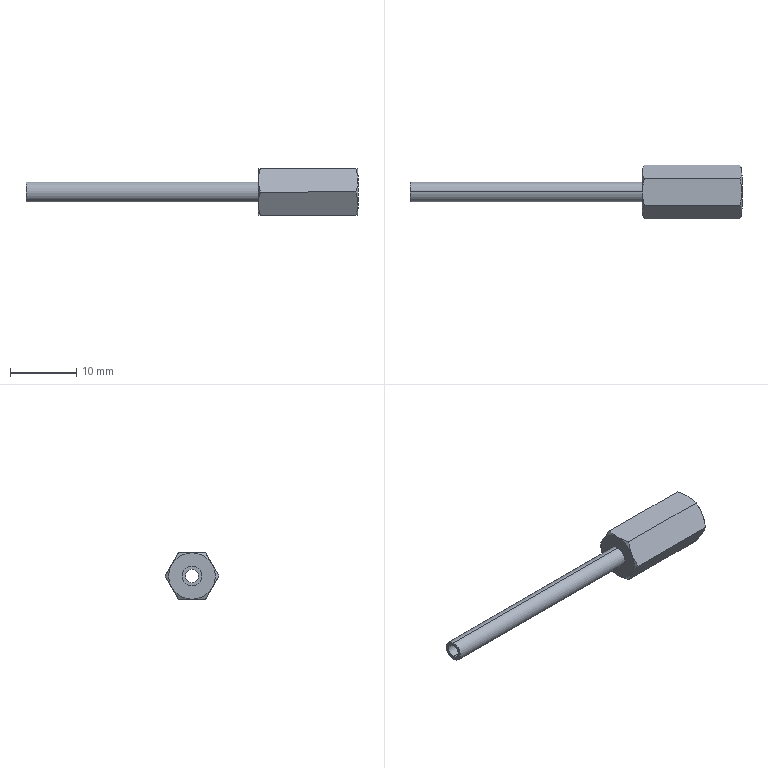Part | SolidWorks | features BaseBody 1 | 1 solid | 31 faces | box 50 x 8.083 x 7 mm | volume 663.119 mm3 | cone 15 | plane 10 | cylinder 6 | commonest cylinder face diameters 2 x2 3 x2 4.134 x2
STEP:
#1=CARTESIAN_POINT('',(0.,0.,1.5));
#2=VERTEX_POINT('',#1);
#3=CARTESIAN_POINT('',(0.,0.,-1.5));
#4=VERTEX_POINT('',#3);
#5=CARTESIAN_POINT('',(0.,0.,0.));
#6=DIRECTION('',(-1.,0.,0.));
#7=DIRECTION('',(0.,0.,1.));
#8=AXIS2_PLACEMENT_3D('',#5,#6,#7);
#9=CIRCLE('',#8,1.5);
#10=EDGE_CURVE('',#2,#4,#9,.T.);
#11=ORIENTED_EDGE('',*,*,#10,.T.);
#12=CARTESIAN_POINT('',(-35.,0.,-1.5));
#13=VERTEX_POINT('',#12);
#14=CARTESIAN_POINT('',(15.,0.,-1.5));
#15=DIRECTION('',(-1.,0.,0.));
#16=VECTOR('',#15,1000.);
#17=LINE('',#14,#16);
#18=EDGE_CURVE('',#4,#13,#17,.T.);
#19=ORIENTED_EDGE('',*,*,#18,.T.);
#20=CARTESIAN_POINT('',(-35.,0.,1.5));
#21=VERTEX_POINT('',#20);
#22=CARTESIAN_POINT('',(-35.,0.,0.));
#23=DIRECTION('',(1.,0.,0.));
#24=DIRECTION('',(0.,0.,1.));
#25=AXIS2_PLACEMENT_3D('',#22,#23,#24);
#26=CIRCLE('',#25,1.5);
#27=EDGE_CURVE('',#13,#21,#26,.T.);
#28=ORIENTED_EDGE('',*,*,#27,.T.);
#29=CARTESIAN_POINT('',(15.,0.,1.5));
#30=DIRECTION('',(-1.,0.,0.));
#31=VECTOR('',#30,1000.);
#32=LINE('',#29,#31);
#33=EDGE_CURVE('',#2,#21,#32,.T.);
#34=ORIENTED_EDGE('',*,*,#33,.F.);
#35=EDGE_LOOP('',(#11,#19,#28,#34));
#36=FACE_OUTER_BOUND('',#35,.T.);
#37=CARTESIAN_POINT('',(15.,0.,0.));
#38=DIRECTION('',(-1.,0.,0.));
#39=DIRECTION('',(0.,0.,1.));
#40=AXIS2_PLACEMENT_3D('',#37,#38,#39);
#41=CYLINDRICAL_SURFACE('',#40,1.5);
#42=ADVANCED_FACE('',(#36),#41,.T.);
#43=CARTESIAN_POINT('',(9.,0.,-1.));
#44=VERTEX_POINT('',#43);
#45=CARTESIAN_POINT('',(9.,0.,1.));
#46=VERTEX_POINT('',#45);
#47=CARTESIAN_POINT('',(9.,0.,0.));
#48=DIRECTION('',(-1.,0.,0.));
#49=DIRECTION('',(0.,0.,1.));
#50=AXIS2_PLACEMENT_3D('',#47,#48,#49);
#51=CIRCLE('',#50,1.);
#52=EDGE_CURVE('',#44,#46,#51,.T.);
#53=ORIENTED_EDGE('',*,*,#52,.F.);
#54=CARTESIAN_POINT('',(-35.,0.,-1.));
#55=VERTEX_POINT('',#54);
#56=CARTESIAN_POINT('',(15.,0.,-1.));
#57=DIRECTION('',(-1.,0.,0.));
#58=VECTOR('',#57,1000.);
#59=LINE('',#56,#58);
#60=EDGE_CURVE('',#44,#55,#59,.T.);
#61=ORIENTED_EDGE('',*,*,#60,.T.);
#62=CARTESIAN_POINT('',(-35.,0.,1.));
#63=VERTEX_POINT('',#62);
#64=CARTESIAN_POINT('',(-35.,0.,0.));
#65=DIRECTION('',(1.,0.,0.));
#66=DIRECTION('',(0.,0.,1.));
#67=AXIS2_PLACEMENT_3D('',#64,#65,#66);
#68=CIRCLE('',#67,1.);
#69=EDGE_CURVE('',#63,#55,#68,.T.);
#70=ORIENTED_EDGE('',*,*,#69,.F.);
#71=CARTESIAN_POINT('',(15.,0.,1.));
#72=DIRECTION('',(-1.,0.,0.));
#73=VECTOR('',#72,1000.);
#74=LINE('',#71,#73);
#75=EDGE_CURVE('',#46,#63,#74,.T.);
#76=ORIENTED_EDGE('',*,*,#75,.F.);
#77=EDGE_LOOP('',(#53,#61,#70,#76));
#78=FACE_OUTER_BOUND('',#77,.T.);
#79=CARTESIAN_POINT('',(15.,0.,0.));
#80=DIRECTION('',(-1.,0.,0.));
#81=DIRECTION('',(0.,0.,1.));
#82=AXIS2_PLACEMENT_3D('',#79,#80,#81);
#83=CYLINDRICAL_SURFACE('',#82,1.);
#84=ADVANCED_FACE('',(#78),#83,.F.);
#85=CARTESIAN_POINT('',(15.,-3.031,-1.75));
#86=VERTEX_POINT('',#85);
#87=CARTESIAN_POINT('',(15.,-3.5,0.));
#88=VERTEX_POINT('',#87);
#89=CARTESIAN_POINT('',(15.,0.,0.));
#90=DIRECTION('',(-1.,0.,0.));
#91=DIRECTION('',(0.,-1.,0.));
#92=AXIS2_PLACEMENT_3D('',#89,#90,#91);
#93=CIRCLE('',#92,3.5);
#94=EDGE_CURVE('',#86,#88,#93,.T.);
#95=ORIENTED_EDGE('',*,*,#94,.T.);
#96=CARTESIAN_POINT('',(14.687,-4.041,0.));
#97=VERTEX_POINT('',#96);
#98=CARTESIAN_POINT('',(14.686,-4.045,0.));
#99=DIRECTION('',(-0.5,-0.866,0.));
#100=VECTOR('',#99,1000.);
#101=LINE('',#98,#100);
#102=EDGE_CURVE('',#88,#97,#101,.T.);
#103=ORIENTED_EDGE('',*,*,#102,.T.);
#104=CARTESIAN_POINT('',(14.687,-4.041,0.));
#105=CARTESIAN_POINT('',(14.878,-3.711,-0.5718));
#106=CARTESIAN_POINT('',(15.,-3.376,-1.153));
#107=CARTESIAN_POINT('',(15.,-3.031,-1.75));
#108=B_SPLINE_CURVE_WITH_KNOTS('',3,(#104,#105,#106,#107),.UNSPECIFIED.,.F.,.F.,(4,4),(0.,0.002045),.UNSPECIFIED.);
#109=EDGE_CURVE('',#97,#86,#108,.T.);
#110=ORIENTED_EDGE('',*,*,#109,.T.);
#111=EDGE_LOOP('',(#95,#103,#110));
#112=FACE_OUTER_BOUND('',#111,.T.);
#113=CARTESIAN_POINT('',(14.686,0.,0.));
#114=DIRECTION('',(-1.,0.,0.));
#115=DIRECTION('',(0.,-1.,0.));
#116=AXIS2_PLACEMENT_3D('',#113,#114,#115);
#117=CONICAL_SURFACE('',#116,4.045,1.047);
#118=ADVANCED_FACE('',(#112),#117,.T.);
#119=CARTESIAN_POINT('',(14.567,0.,-2.067));
#120=VERTEX_POINT('',#119);
#121=CARTESIAN_POINT('',(14.567,-2.067,0.));
#122=VERTEX_POINT('',#121);
#123=CARTESIAN_POINT('',(14.567,0.,0.));
#124=DIRECTION('',(-1.,0.,0.));
#125=DIRECTION('',(0.,0.,1.));
#126=AXIS2_PLACEMENT_3D('',#123,#124,#125);
#127=CIRCLE('',#126,2.067);
#128=EDGE_CURVE('',#120,#122,#127,.T.);
#129=ORIENTED_EDGE('',*,*,#128,.F.);
#130=CARTESIAN_POINT('',(9.,0.,-2.067));
#131=VERTEX_POINT('',#130);
#132=CARTESIAN_POINT('',(15.,0.,-2.067));
#133=DIRECTION('',(-1.,0.,0.));
#134=VECTOR('',#133,1000.);
#135=LINE('',#132,#134);
#136=EDGE_CURVE('',#120,#131,#135,.T.);
#137=ORIENTED_EDGE('',*,*,#136,.T.);
#138=CARTESIAN_POINT('',(9.,0.,2.067));
#139=VERTEX_POINT('',#138);
#140=CARTESIAN_POINT('',(9.,0.,0.));
#141=DIRECTION('',(1.,0.,0.));
#142=DIRECTION('',(0.,0.,1.));
#143=AXIS2_PLACEMENT_3D('',#140,#141,#142);
#144=CIRCLE('',#143,2.067);
#145=EDGE_CURVE('',#139,#131,#144,.T.);
#146=ORIENTED_EDGE('',*,*,#145,.F.);
#147=CARTESIAN_POINT('',(14.567,0.,2.067));
#148=VERTEX_POINT('',#147);
#149=CARTESIAN_POINT('',(15.,0.,2.067));
#150=DIRECTION('',(-1.,0.,0.));
#151=VECTOR('',#150,1000.);
#152=LINE('',#149,#151);
#153=EDGE_CURVE('',#148,#139,#152,.T.);
#154=ORIENTED_EDGE('',*,*,#153,.F.);
#155=CARTESIAN_POINT('',(14.567,0.,0.));
#156=DIRECTION('',(-1.,0.,0.));
#157=DIRECTION('',(0.,0.,1.));
#158=AXIS2_PLACEMENT_3D('',#155,#156,#157);
#159=CIRCLE('',#158,2.067);
#160=EDGE_CURVE('',#122,#148,#159,.T.);
#161=ORIENTED_EDGE('',*,*,#160,.F.);
#162=EDGE_LOOP('',(#129,#137,#146,#154,#161));
#163=FACE_OUTER_BOUND('',#162,.T.);
#164=CARTESIAN_POINT('',(15.,0.,0.));
#165=DIRECTION('',(-1.,0.,0.));
#166=DIRECTION('',(0.,0.,1.));
#167=AXIS2_PLACEMENT_3D('',#164,#165,#166);
#168=CYLINDRICAL_SURFACE('',#167,2.067);
#169=ADVANCED_FACE('',(#163),#168,.F.);
#170=CARTESIAN_POINT('',(14.567,2.067,0.));
#171=VERTEX_POINT('',#170);
#172=CARTESIAN_POINT('',(14.567,0.,0.));
#173=DIRECTION('',(-1.,0.,0.));
#174=DIRECTION('',(0.,0.,1.));
#175=AXIS2_PLACEMENT_3D('',#172,#173,#174);
#176=CIRCLE('',#175,2.067);
#177=EDGE_CURVE('',#171,#120,#176,.T.);
#178=ORIENTED_EDGE('',*,*,#177,.T.);
#179=ORIENTED_EDGE('',*,*,#128,.T.);
#180=CARTESIAN_POINT('',(15.,-2.5,0.));
#181=VERTEX_POINT('',#180);
#182=CARTESIAN_POINT('',(15.,-2.5,0.));
#183=DIRECTION('',(0.7071,-0.7071,0.));
#184=VECTOR('',#183,1000.);
#185=LINE('',#182,#184);
#186=EDGE_CURVE('',#122,#181,#185,.T.);
#187=ORIENTED_EDGE('',*,*,#186,.T.);
#188=CARTESIAN_POINT('',(15.,2.5,0.));
#189=VERTEX_POINT('',#188);
#190=CARTESIAN_POINT('',(15.,0.,0.));
#191=DIRECTION('',(-1.,0.,0.));
#192=DIRECTION('',(0.,1.,0.));
#193=AXIS2_PLACEMENT_3D('',#190,#191,#192);
#194=CIRCLE('',#193,2.5);
#195=EDGE_CURVE('',#189,#181,#194,.T.);
#196=ORIENTED_EDGE('',*,*,#195,.F.);
#197=CARTESIAN_POINT('',(15.,2.5,0.));
#198=DIRECTION('',(0.7071,0.7071,0.));
#199=VECTOR('',#198,1000.);
#200=LINE('',#197,#199);
#201=EDGE_CURVE('',#171,#189,#200,.T.);
#202=ORIENTED_EDGE('',*,*,#201,.F.);
#203=EDGE_LOOP('',(#178,#179,#187,#196,#202));
#204=FACE_OUTER_BOUND('',#203,.T.);
#205=CARTESIAN_POINT('',(15.,0.,0.));
#206=DIRECTION('',(1.,0.,0.));
#207=DIRECTION('',(0.,1.,0.));
#208=AXIS2_PLACEMENT_3D('',#205,#206,#207);
#209=CONICAL_SURFACE('',#208,2.5,0.7854);
#210=ADVANCED_FACE('',(#204),#209,.F.);
#211=ORIENTED_EDGE('',*,*,#18,.F.);
#212=CARTESIAN_POINT('',(0.,0.,0.));
#213=DIRECTION('',(-1.,0.,0.));
#214=DIRECTION('',(0.,0.,1.));
#215=AXIS2_PLACEMENT_3D('',#212,#213,#214);
#216=CIRCLE('',#215,1.5);
#217=EDGE_CURVE('',#4,#2,#216,.T.);
#218=ORIENTED_EDGE('',*,*,#217,.T.);
#219=ORIENTED_EDGE('',*,*,#33,.T.);
#220=CARTESIAN_POINT('',(-35.,0.,0.));
#221=DIRECTION('',(1.,0.,0.));
#222=DIRECTION('',(0.,0.,1.));
#223=AXIS2_PLACEMENT_3D('',#220,#221,#222);
#224=CIRCLE('',#223,1.5);
#225=EDGE_CURVE('',#21,#13,#224,.T.);
#226=ORIENTED_EDGE('',*,*,#225,.T.);
#227=EDGE_LOOP('',(#211,#218,#219,#226));
#228=FACE_OUTER_BOUND('',#227,.T.);
#229=CARTESIAN_POINT('',(15.,0.,0.));
#230=DIRECTION('',(-1.,0.,0.));
#231=DIRECTION('',(0.,0.,1.));
#232=AXIS2_PLACEMENT_3D('',#229,#230,#231);
#233=CYLINDRICAL_SURFACE('',#232,1.5);
#234=ADVANCED_FACE('',(#228),#233,.T.);
#235=CARTESIAN_POINT('',(0.,-3.031,1.75));
#236=VERTEX_POINT('',#235);
#237=CARTESIAN_POINT('',(0.,0.,3.5));
#238=VERTEX_POINT('',#237);
#239=CARTESIAN_POINT('',(0.,0.,0.));
#240=DIRECTION('',(-1.,0.,0.));
#241=DIRECTION('',(0.,0.,-1.));
#242=AXIS2_PLACEMENT_3D('',#239,#240,#241);
#243=CIRCLE('',#242,3.5);
#244=EDGE_CURVE('',#236,#238,#243,.T.);
#245=ORIENTED_EDGE('',*,*,#244,.T.);
#246=CARTESIAN_POINT('',(0.,3.031,1.75));
#247=VERTEX_POINT('',#246);
#248=CARTESIAN_POINT('',(0.,0.,0.));
#249=DIRECTION('',(-1.,0.,0.));
#250=DIRECTION('',(0.,0.,-1.));
#251=AXIS2_PLACEMENT_3D('',#248,#249,#250);
#252=CIRCLE('',#251,3.5);
#253=EDGE_CURVE('',#238,#247,#252,.T.);
#254=ORIENTED_EDGE('',*,*,#253,.T.);
#255=CARTESIAN_POINT('',(0.,3.031,-1.75));
#256=VERTEX_POINT('',#255);
#257=CARTESIAN_POINT('',(0.,0.,0.));
#258=DIRECTION('',(-1.,0.,0.));
#259=DIRECTION('',(0.,0.,-1.));
#260=AXIS2_PLACEMENT_3D('',#257,#258,#259);
#261=CIRCLE('',#260,3.5);
#262=EDGE_CURVE('',#247,#256,#261,.T.);
#263=ORIENTED_EDGE('',*,*,#262,.T.);
#264=CARTESIAN_POINT('',(0.,0.,-3.5));
#265=VERTEX_POINT('',#264);
#266=CARTESIAN_POINT('',(0.,0.,0.));
#267=DIRECTION('',(-1.,0.,0.));
#268=DIRECTION('',(0.,0.,-1.));
#269=AXIS2_PLACEMENT_3D('',#266,#267,#268);
#270=CIRCLE('',#269,3.5);
#271=EDGE_CURVE('',#256,#265,#270,.T.);
#272=ORIENTED_EDGE('',*,*,#271,.T.);
#273=CARTESIAN_POINT('',(0.,-3.031,-1.75));
#274=VERTEX_POINT('',#273);
#275=CARTESIAN_POINT('',(0.,0.,0.));
#276=DIRECTION('',(-1.,0.,0.));
#277=DIRECTION('',(0.,0.,-1.));
#278=AXIS2_PLACEMENT_3D('',#275,#276,#277);
#279=CIRCLE('',#278,3.5);
#280=EDGE_CURVE('',#265,#274,#279,.T.);
#281=ORIENTED_EDGE('',*,*,#280,.T.);
#282=CARTESIAN_POINT('',(0.,0.,0.));
#283=DIRECTION('',(-1.,0.,0.));
#284=DIRECTION('',(0.,0.,-1.));
#285=AXIS2_PLACEMENT_3D('',#282,#283,#284);
#286=CIRCLE('',#285,3.5);
#287=EDGE_CURVE('',#274,#236,#286,.T.);
#288=ORIENTED_EDGE('',*,*,#287,.T.);
#289=EDGE_LOOP('',(#245,#254,#263,#272,#281,#288));
#290=FACE_OUTER_BOUND('',#289,.T.);
#291=ORIENTED_EDGE('',*,*,#10,.F.);
#292=ORIENTED_EDGE('',*,*,#217,.F.);
#293=EDGE_LOOP('',(#291,#292));
#294=FACE_BOUND('',#293,.T.);
#295=CARTESIAN_POINT('',(0.,3.5,0.));
#296=DIRECTION('',(-1.,0.,0.));
#297=DIRECTION('',(0.,0.,1.));
#298=AXIS2_PLACEMENT_3D('',#295,#296,#297);
#299=PLANE('',#298);
#300=ADVANCED_FACE('',(#290,#294),#299,.T.);
#301=ORIENTED_EDGE('',*,*,#225,.F.);
#302=ORIENTED_EDGE('',*,*,#27,.F.);
#303=EDGE_LOOP('',(#301,#302));
#304=FACE_OUTER_BOUND('',#303,.T.);
#305=ORIENTED_EDGE('',*,*,#69,.T.);
#306=CARTESIAN_POINT('',(-35.,0.,0.));
#307=DIRECTION('',(1.,0.,0.));
#308=DIRECTION('',(0.,0.,1.));
#309=AXIS2_PLACEMENT_3D('',#306,#307,#308);
#310=CIRCLE('',#309,1.);
#311=EDGE_CURVE('',#55,#63,#310,.T.);
#312=ORIENTED_EDGE('',*,*,#311,.T.);
#313=EDGE_LOOP('',(#305,#312));
#314=FACE_BOUND('',#313,.T.);
#315=CARTESIAN_POINT('',(-35.,1.5,0.));
#316=DIRECTION('',(-1.,0.,0.));
#317=DIRECTION('',(0.,0.,1.));
#318=AXIS2_PLACEMENT_3D('',#315,#316,#317);
#319=PLANE('',#318);
#320=ADVANCED_FACE('',(#304,#314),#319,.T.);
#321=ORIENTED_EDGE('',*,*,#253,.F.);
#322=CARTESIAN_POINT('',(0.3126,2.021,3.5));
#323=VERTEX_POINT('',#322);
#324=CARTESIAN_POINT('',(0.,0.,3.5));
#325=CARTESIAN_POINT('',(0.,0.6897,3.5));
#326=CARTESIAN_POINT('',(0.122,1.361,3.5));
#327=CARTESIAN_POINT('',(0.3126,2.021,3.5));
#328=B_SPLINE_CURVE_WITH_KNOTS('',3,(#324,#325,#326,#327),.UNSPECIFIED.,.F.,.F.,(4,4),(0.,0.002045),.UNSPECIFIED.);
#329=EDGE_CURVE('',#238,#323,#328,.T.);
#330=ORIENTED_EDGE('',*,*,#329,.T.);
#331=CARTESIAN_POINT('',(0.3126,2.021,3.5));
#332=CARTESIAN_POINT('',(0.122,2.351,2.928));
#333=CARTESIAN_POINT('',(0.,2.686,2.347));
#334=CARTESIAN_POINT('',(0.,3.031,1.75));
#335=B_SPLINE_CURVE_WITH_KNOTS('',3,(#331,#332,#333,#334),.UNSPECIFIED.,.F.,.F.,(4,4),(0.,0.002045),.UNSPECIFIED.);
#336=EDGE_CURVE('',#323,#247,#335,.T.);
#337=ORIENTED_EDGE('',*,*,#336,.T.);
#338=EDGE_LOOP('',(#321,#330,#337));
#339=FACE_OUTER_BOUND('',#338,.T.);
#340=CARTESIAN_POINT('',(0.3145,0.,0.));
#341=DIRECTION('',(1.,0.,0.));
#342=DIRECTION('',(0.,0.,-1.));
#343=AXIS2_PLACEMENT_3D('',#340,#341,#342);
#344=CONICAL_SURFACE('',#343,4.045,1.047);
#345=ADVANCED_FACE('',(#339),#344,.T.);
#346=ORIENTED_EDGE('',*,*,#244,.F.);
#347=CARTESIAN_POINT('',(0.3126,-2.021,3.5));
#348=VERTEX_POINT('',#347);
#349=CARTESIAN_POINT('',(0.,-3.031,1.75));
#350=CARTESIAN_POINT('',(0.,-2.686,2.347));
#351=CARTESIAN_POINT('',(0.122,-2.351,2.928));
#352=CARTESIAN_POINT('',(0.3126,-2.021,3.5));
#353=B_SPLINE_CURVE_WITH_KNOTS('',3,(#349,#350,#351,#352),.UNSPECIFIED.,.F.,.F.,(4,4),(0.,0.002045),.UNSPECIFIED.);
#354=EDGE_CURVE('',#236,#348,#353,.T.);
#355=ORIENTED_EDGE('',*,*,#354,.T.);
#356=CARTESIAN_POINT('',(0.3126,-2.021,3.5));
#357=CARTESIAN_POINT('',(0.122,-1.361,3.5));
#358=CARTESIAN_POINT('',(0.,-0.6897,3.5));
#359=CARTESIAN_POINT('',(0.,0.,3.5));
#360=B_SPLINE_CURVE_WITH_KNOTS('',3,(#356,#357,#358,#359),.UNSPECIFIED.,.F.,.F.,(4,4),(0.,0.002045),.UNSPECIFIED.);
#361=EDGE_CURVE('',#348,#238,#360,.T.);
#362=ORIENTED_EDGE('',*,*,#361,.T.);
#363=EDGE_LOOP('',(#346,#355,#362));
#364=FACE_OUTER_BOUND('',#363,.T.);
#365=CARTESIAN_POINT('',(0.3145,0.,0.));
#366=DIRECTION('',(1.,0.,0.));
#367=DIRECTION('',(0.,0.,-1.));
#368=AXIS2_PLACEMENT_3D('',#365,#366,#367);
#369=CONICAL_SURFACE('',#368,4.045,1.047);
#370=ADVANCED_FACE('',(#364),#369,.T.);
#371=CARTESIAN_POINT('',(0.3126,-4.041,-0.000000014));
#372=VERTEX_POINT('',#371);
#373=CARTESIAN_POINT('',(0.3126,-4.041,-0.000000014));
#374=CARTESIAN_POINT('',(0.122,-3.711,0.5718));
#375=CARTESIAN_POINT('',(0.,-3.376,1.153));
#376=CARTESIAN_POINT('',(0.,-3.031,1.75));
#377=B_SPLINE_CURVE_WITH_KNOTS('',3,(#373,#374,#375,#376),.UNSPECIFIED.,.F.,.F.,(4,4),(0.,0.002045),.UNSPECIFIED.);
#378=EDGE_CURVE('',#372,#236,#377,.T.);
#379=ORIENTED_EDGE('',*,*,#378,.T.);
#380=ORIENTED_EDGE('',*,*,#287,.F.);
#381=CARTESIAN_POINT('',(0.,-3.031,-1.75));
#382=CARTESIAN_POINT('',(0.,-3.376,-1.153));
#383=CARTESIAN_POINT('',(0.122,-3.711,-0.5718));
#384=CARTESIAN_POINT('',(0.3126,-4.041,-0.000000014));
#385=B_SPLINE_CURVE_WITH_KNOTS('',3,(#381,#382,#383,#384),.UNSPECIFIED.,.F.,.F.,(4,4),(0.,0.002045),.UNSPECIFIED.);
#386=EDGE_CURVE('',#274,#372,#385,.T.);
#387=ORIENTED_EDGE('',*,*,#386,.T.);
#388=EDGE_LOOP('',(#379,#380,#387));
#389=FACE_OUTER_BOUND('',#388,.T.);
#390=CARTESIAN_POINT('',(0.3145,0.,0.));
#391=DIRECTION('',(1.,0.,0.));
#392=DIRECTION('',(0.,0.,-1.));
#393=AXIS2_PLACEMENT_3D('',#390,#391,#392);
#394=CONICAL_SURFACE('',#393,4.045,1.047);
#395=ADVANCED_FACE('',(#389),#394,.T.);
#396=CARTESIAN_POINT('',(0.3126,-2.021,-3.5));
#397=VERTEX_POINT('',#396);
#398=CARTESIAN_POINT('',(0.3126,-2.021,-3.5));
#399=CARTESIAN_POINT('',(0.122,-2.351,-2.928));
#400=CARTESIAN_POINT('',(0.,-2.686,-2.347));
#401=CARTESIAN_POINT('',(0.,-3.031,-1.75));
#402=B_SPLINE_CURVE_WITH_KNOTS('',3,(#398,#399,#400,#401),.UNSPECIFIED.,.F.,.F.,(4,4),(0.,0.002045),.UNSPECIFIED.);
#403=EDGE_CURVE('',#397,#274,#402,.T.);
#404=ORIENTED_EDGE('',*,*,#403,.T.);
#405=ORIENTED_EDGE('',*,*,#280,.F.);
#406=CARTESIAN_POINT('',(0.,0.,-3.5));
#407=CARTESIAN_POINT('',(0.,-0.6897,-3.5));
#408=CARTESIAN_POINT('',(0.122,-1.361,-3.5));
#409=CARTESIAN_POINT('',(0.3126,-2.021,-3.5));
#410=B_SPLINE_CURVE_WITH_KNOTS('',3,(#406,#407,#408,#409),.UNSPECIFIED.,.F.,.F.,(4,4),(0.,0.002045),.UNSPECIFIED.);
#411=EDGE_CURVE('',#265,#397,#410,.T.);
#412=ORIENTED_EDGE('',*,*,#411,.T.);
#413=EDGE_LOOP('',(#404,#405,#412));
#414=FACE_OUTER_BOUND('',#413,.T.);
#415=CARTESIAN_POINT('',(0.3145,0.,0.));
#416=DIRECTION('',(1.,0.,0.));
#417=DIRECTION('',(0.,0.,-1.));
#418=AXIS2_PLACEMENT_3D('',#415,#416,#417);
#419=CONICAL_SURFACE('',#418,4.045,1.047);
#420=ADVANCED_FACE('',(#414),#419,.T.);
#421=CARTESIAN_POINT('',(0.3126,2.021,-3.5));
#422=VERTEX_POINT('',#421);
#423=CARTESIAN_POINT('',(0.3126,2.021,-3.5));
#424=CARTESIAN_POINT('',(0.122,1.361,-3.5));
#425=CARTESIAN_POINT('',(0.,0.6897,-3.5));
#426=CARTESIAN_POINT('',(0.,0.,-3.5));
#427=B_SPLINE_CURVE_WITH_KNOTS('',3,(#423,#424,#425,#426),.UNSPECIFIED.,.F.,.F.,(4,4),(0.,0.002045),.UNSPECIFIED.);
#428=EDGE_CURVE('',#422,#265,#427,.T.);
#429=ORIENTED_EDGE('',*,*,#428,.T.);
#430=ORIENTED_EDGE('',*,*,#271,.F.);
#431=CARTESIAN_POINT('',(0.,3.031,-1.75));
#432=CARTESIAN_POINT('',(0.,2.686,-2.347));
#433=CARTESIAN_POINT('',(0.122,2.351,-2.928));
#434=CARTESIAN_POINT('',(0.3126,2.021,-3.5));
#435=B_SPLINE_CURVE_WITH_KNOTS('',3,(#431,#432,#433,#434),.UNSPECIFIED.,.F.,.F.,(4,4),(0.,0.002045),.UNSPECIFIED.);
#436=EDGE_CURVE('',#256,#422,#435,.T.);
#437=ORIENTED_EDGE('',*,*,#436,.T.);
#438=EDGE_LOOP('',(#429,#430,#437));
#439=FACE_OUTER_BOUND('',#438,.T.);
#440=CARTESIAN_POINT('',(0.3145,0.,0.));
#441=DIRECTION('',(1.,0.,0.));
#442=DIRECTION('',(0.,0.,-1.));
#443=AXIS2_PLACEMENT_3D('',#440,#441,#442);
#444=CONICAL_SURFACE('',#443,4.045,1.047);
#445=ADVANCED_FACE('',(#439),#444,.T.);
#446=CARTESIAN_POINT('',(0.3126,4.041,0.000000014));
#447=VERTEX_POINT('',#446);
#448=CARTESIAN_POINT('',(0.3126,4.041,0.000000014));
#449=CARTESIAN_POINT('',(0.122,3.711,-0.5718));
#450=CARTESIAN_POINT('',(0.,3.376,-1.153));
#451=CARTESIAN_POINT('',(0.,3.031,-1.75));
#452=B_SPLINE_CURVE_WITH_KNOTS('',3,(#448,#449,#450,#451),.UNSPECIFIED.,.F.,.F.,(4,4),(0.,0.002045),.UNSPECIFIED.);
#453=EDGE_CURVE('',#447,#256,#452,.T.);
#454=ORIENTED_EDGE('',*,*,#453,.T.);
#455=ORIENTED_EDGE('',*,*,#262,.F.);
#456=CARTESIAN_POINT('',(0.,3.031,1.75));
#457=CARTESIAN_POINT('',(0.,3.376,1.153));
#458=CARTESIAN_POINT('',(0.122,3.711,0.5718));
#459=CARTESIAN_POINT('',(0.3126,4.041,0.000000014));
#460=B_SPLINE_CURVE_WITH_KNOTS('',3,(#456,#457,#458,#459),.UNSPECIFIED.,.F.,.F.,(4,4),(0.,0.002045),.UNSPECIFIED.);
#461=EDGE_CURVE('',#247,#447,#460,.T.);
#462=ORIENTED_EDGE('',*,*,#461,.T.);
#463=EDGE_LOOP('',(#454,#455,#462));
#464=FACE_OUTER_BOUND('',#463,.T.);
#465=CARTESIAN_POINT('',(0.3145,0.,0.));
#466=DIRECTION('',(1.,0.,0.));
#467=DIRECTION('',(0.,0.,-1.));
#468=AXIS2_PLACEMENT_3D('',#465,#466,#467);
#469=CONICAL_SURFACE('',#468,4.045,1.047);
#470=ADVANCED_FACE('',(#464),#469,.T.);
#471=ORIENTED_EDGE('',*,*,#60,.F.);
#472=CARTESIAN_POINT('',(9.,0.,0.));
#473=DIRECTION('',(-1.,0.,0.));
#474=DIRECTION('',(0.,0.,1.));
#475=AXIS2_PLACEMENT_3D('',#472,#473,#474);
#476=CIRCLE('',#475,1.);
#477=EDGE_CURVE('',#46,#44,#476,.T.);
#478=ORIENTED_EDGE('',*,*,#477,.F.);
#479=ORIENTED_EDGE('',*,*,#75,.T.);
#480=ORIENTED_EDGE('',*,*,#311,.F.);
#481=EDGE_LOOP('',(#471,#478,#479,#480));
#482=FACE_OUTER_BOUND('',#481,.T.);
#483=CARTESIAN_POINT('',(15.,0.,0.));
#484=DIRECTION('',(-1.,0.,0.));
#485=DIRECTION('',(0.,0.,1.));
#486=AXIS2_PLACEMENT_3D('',#483,#484,#485);
#487=CYLINDRICAL_SURFACE('',#486,1.);
#488=ADVANCED_FACE('',(#482),#487,.F.);
#489=CARTESIAN_POINT('',(14.687,2.021,3.5));
#490=VERTEX_POINT('',#489);
#491=CARTESIAN_POINT('',(15.,0.,3.5));
#492=VERTEX_POINT('',#491);
#493=CARTESIAN_POINT('',(14.687,2.021,3.5));
#494=CARTESIAN_POINT('',(14.878,1.361,3.5));
#495=CARTESIAN_POINT('',(15.,0.6897,3.5));
#496=CARTESIAN_POINT('',(15.,0.,3.5));
#497=B_SPLINE_CURVE_WITH_KNOTS('',3,(#493,#494,#495,#496),.UNSPECIFIED.,.F.,.F.,(4,4),(0.,0.002045),.UNSPECIFIED.);
#498=EDGE_CURVE('',#490,#492,#497,.T.);
#499=ORIENTED_EDGE('',*,*,#498,.F.);
#500=CARTESIAN_POINT('',(23.,2.021,3.5));
#501=DIRECTION('',(1.,0.,0.));
#502=VECTOR('',#501,1000.);
#503=LINE('',#500,#502);
#504=EDGE_CURVE('',#323,#490,#503,.T.);
#505=ORIENTED_EDGE('',*,*,#504,.F.);
#506=ORIENTED_EDGE('',*,*,#329,.F.);
#507=ORIENTED_EDGE('',*,*,#361,.F.);
#508=CARTESIAN_POINT('',(14.687,-2.021,3.5));
#509=VERTEX_POINT('',#508);
#510=CARTESIAN_POINT('',(23.,-2.021,3.5));
#511=DIRECTION('',(-1.,0.,0.));
#512=VECTOR('',#511,1000.);
#513=LINE('',#510,#512);
#514=EDGE_CURVE('',#509,#348,#513,.T.);
#515=ORIENTED_EDGE('',*,*,#514,.F.);
#516=CARTESIAN_POINT('',(15.,0.,3.5));
#517=CARTESIAN_POINT('',(15.,-0.6897,3.5));
#518=CARTESIAN_POINT('',(14.878,-1.361,3.5));
#519=CARTESIAN_POINT('',(14.687,-2.021,3.5));
#520=B_SPLINE_CURVE_WITH_KNOTS('',3,(#516,#517,#518,#519),.UNSPECIFIED.,.F.,.F.,(4,4),(0.,0.002045),.UNSPECIFIED.);
#521=EDGE_CURVE('',#492,#509,#520,.T.);
#522=ORIENTED_EDGE('',*,*,#521,.F.);
#523=EDGE_LOOP('',(#499,#505,#506,#507,#515,#522));
#524=FACE_OUTER_BOUND('',#523,.T.);
#525=CARTESIAN_POINT('',(23.,2.021,3.5));
#526=DIRECTION('',(0.,0.,-1.));
#527=DIRECTION('',(-1.,0.,0.));
#528=AXIS2_PLACEMENT_3D('',#525,#526,#527);
#529=PLANE('',#528);
#530=ADVANCED_FACE('',(#524),#529,.F.);
#531=CARTESIAN_POINT('',(14.687,4.041,0.));
#532=VERTEX_POINT('',#531);
#533=CARTESIAN_POINT('',(15.,3.031,1.75));
#534=VERTEX_POINT('',#533);
#535=CARTESIAN_POINT('',(14.687,4.041,0.));
#536=CARTESIAN_POINT('',(14.878,3.711,0.5718));
#537=CARTESIAN_POINT('',(15.,3.376,1.153));
#538=CARTESIAN_POINT('',(15.,3.031,1.75));
#539=B_SPLINE_CURVE_WITH_KNOTS('',3,(#535,#536,#537,#538),.UNSPECIFIED.,.F.,.F.,(4,4),(0.,0.002045),.UNSPECIFIED.);
#540=EDGE_CURVE('',#532,#534,#539,.T.);
#541=ORIENTED_EDGE('',*,*,#540,.F.);
#542=CARTESIAN_POINT('',(23.,4.041,0.));
#543=DIRECTION('',(1.,0.,0.));
#544=VECTOR('',#543,1000.);
#545=LINE('',#542,#544);
#546=EDGE_CURVE('',#447,#532,#545,.T.);
#547=ORIENTED_EDGE('',*,*,#546,.F.);
#548=ORIENTED_EDGE('',*,*,#461,.F.);
#549=ORIENTED_EDGE('',*,*,#336,.F.);
#550=ORIENTED_EDGE('',*,*,#504,.T.);
#551=CARTESIAN_POINT('',(15.,3.031,1.75));
#552=CARTESIAN_POINT('',(15.,2.686,2.347));
#553=CARTESIAN_POINT('',(14.878,2.351,2.928));
#554=CARTESIAN_POINT('',(14.687,2.021,3.5));
#555=B_SPLINE_CURVE_WITH_KNOTS('',3,(#551,#552,#553,#554),.UNSPECIFIED.,.F.,.F.,(4,4),(0.,0.002045),.UNSPECIFIED.);
#556=EDGE_CURVE('',#534,#490,#555,.T.);
#557=ORIENTED_EDGE('',*,*,#556,.F.);
#558=EDGE_LOOP('',(#541,#547,#548,#549,#550,#557));
#559=FACE_OUTER_BOUND('',#558,.T.);
#560=CARTESIAN_POINT('',(23.,4.041,0.));
#561=DIRECTION('',(0.,-0.866,-0.5));
#562=DIRECTION('',(0.,0.5,-0.866));
#563=AXIS2_PLACEMENT_3D('',#560,#561,#562);
#564=PLANE('',#563);
#565=ADVANCED_FACE('',(#559),#564,.F.);
#566=CARTESIAN_POINT('',(15.,-3.031,1.75));
#567=VERTEX_POINT('',#566);
#568=CARTESIAN_POINT('',(14.687,-2.021,3.5));
#569=CARTESIAN_POINT('',(14.878,-2.351,2.928));
#570=CARTESIAN_POINT('',(15.,-2.686,2.347));
#571=CARTESIAN_POINT('',(15.,-3.031,1.75));
#572=B_SPLINE_CURVE_WITH_KNOTS('',3,(#568,#569,#570,#571),.UNSPECIFIED.,.F.,.F.,(4,4),(0.,0.002045),.UNSPECIFIED.);
#573=EDGE_CURVE('',#509,#567,#572,.T.);
#574=ORIENTED_EDGE('',*,*,#573,.F.);
#575=ORIENTED_EDGE('',*,*,#514,.T.);
#576=ORIENTED_EDGE('',*,*,#354,.F.);
#577=ORIENTED_EDGE('',*,*,#378,.F.);
#578=CARTESIAN_POINT('',(23.,-4.041,0.));
#579=DIRECTION('',(-1.,0.,0.));
#580=VECTOR('',#579,1000.);
#581=LINE('',#578,#580);
#582=EDGE_CURVE('',#97,#372,#581,.T.);
#583=ORIENTED_EDGE('',*,*,#582,.F.);
#584=CARTESIAN_POINT('',(15.,-3.031,1.75));
#585=CARTESIAN_POINT('',(15.,-3.376,1.153));
#586=CARTESIAN_POINT('',(14.878,-3.711,0.5718));
#587=CARTESIAN_POINT('',(14.687,-4.041,0.));
#588=B_SPLINE_CURVE_WITH_KNOTS('',3,(#584,#585,#586,#587),.UNSPECIFIED.,.F.,.F.,(4,4),(0.,0.002045),.UNSPECIFIED.);
#589=EDGE_CURVE('',#567,#97,#588,.T.);
#590=ORIENTED_EDGE('',*,*,#589,.F.);
#591=EDGE_LOOP('',(#574,#575,#576,#577,#583,#590));
#592=FACE_OUTER_BOUND('',#591,.T.);
#593=CARTESIAN_POINT('',(23.,-2.021,3.5));
#594=DIRECTION('',(0.,0.866,-0.5));
#595=DIRECTION('',(0.,0.5,0.866));
#596=AXIS2_PLACEMENT_3D('',#593,#594,#595);
#597=PLANE('',#596);
#598=ADVANCED_FACE('',(#592),#597,.F.);
#599=ORIENTED_EDGE('',*,*,#109,.F.);
#600=ORIENTED_EDGE('',*,*,#582,.T.);
#601=ORIENTED_EDGE('',*,*,#386,.F.);
#602=ORIENTED_EDGE('',*,*,#403,.F.);
#603=CARTESIAN_POINT('',(14.687,-2.021,-3.5));
#604=VERTEX_POINT('',#603);
#605=CARTESIAN_POINT('',(23.,-2.021,-3.5));
#606=DIRECTION('',(-1.,0.,0.));
#607=VECTOR('',#606,1000.);
#608=LINE('',#605,#607);
#609=EDGE_CURVE('',#604,#397,#608,.T.);
#610=ORIENTED_EDGE('',*,*,#609,.F.);
#611=CARTESIAN_POINT('',(15.,-3.031,-1.75));
#612=CARTESIAN_POINT('',(15.,-2.686,-2.347));
#613=CARTESIAN_POINT('',(14.878,-2.351,-2.928));
#614=CARTESIAN_POINT('',(14.687,-2.021,-3.5));
#615=B_SPLINE_CURVE_WITH_KNOTS('',3,(#611,#612,#613,#614),.UNSPECIFIED.,.F.,.F.,(4,4),(0.,0.002045),.UNSPECIFIED.);
#616=EDGE_CURVE('',#86,#604,#615,.T.);
#617=ORIENTED_EDGE('',*,*,#616,.F.);
#618=EDGE_LOOP('',(#599,#600,#601,#602,#610,#617));
#619=FACE_OUTER_BOUND('',#618,.T.);
#620=CARTESIAN_POINT('',(23.,-4.041,0.));
#621=DIRECTION('',(0.,0.866,0.5));
#622=DIRECTION('',(0.,-0.5,0.866));
#623=AXIS2_PLACEMENT_3D('',#620,#621,#622);
#624=PLANE('',#623);
#625=ADVANCED_FACE('',(#619),#624,.F.);
#626=CARTESIAN_POINT('',(15.,0.,-3.5));
#627=VERTEX_POINT('',#626);
#628=CARTESIAN_POINT('',(14.687,-2.021,-3.5));
#629=CARTESIAN_POINT('',(14.878,-1.361,-3.5));
#630=CARTESIAN_POINT('',(15.,-0.6897,-3.5));
#631=CARTESIAN_POINT('',(15.,0.,-3.5));
#632=B_SPLINE_CURVE_WITH_KNOTS('',3,(#628,#629,#630,#631),.UNSPECIFIED.,.F.,.F.,(4,4),(0.,0.002045),.UNSPECIFIED.);
#633=EDGE_CURVE('',#604,#627,#632,.T.);
#634=ORIENTED_EDGE('',*,*,#633,.F.);
#635=ORIENTED_EDGE('',*,*,#609,.T.);
#636=ORIENTED_EDGE('',*,*,#411,.F.);
#637=ORIENTED_EDGE('',*,*,#428,.F.);
#638=CARTESIAN_POINT('',(14.687,2.021,-3.5));
#639=VERTEX_POINT('',#638);
#640=CARTESIAN_POINT('',(23.,2.021,-3.5));
#641=DIRECTION('',(-1.,0.,0.));
#642=VECTOR('',#641,1000.);
#643=LINE('',#640,#642);
#644=EDGE_CURVE('',#639,#422,#643,.T.);
#645=ORIENTED_EDGE('',*,*,#644,.F.);
#646=CARTESIAN_POINT('',(15.,0.,-3.5));
#647=CARTESIAN_POINT('',(15.,0.6897,-3.5));
#648=CARTESIAN_POINT('',(14.878,1.361,-3.5));
#649=CARTESIAN_POINT('',(14.687,2.021,-3.5));
#650=B_SPLINE_CURVE_WITH_KNOTS('',3,(#646,#647,#648,#649),.UNSPECIFIED.,.F.,.F.,(4,4),(0.,0.002045),.UNSPECIFIED.);
#651=EDGE_CURVE('',#627,#639,#650,.T.);
#652=ORIENTED_EDGE('',*,*,#651,.F.);
#653=EDGE_LOOP('',(#634,#635,#636,#637,#645,#652));
#654=FACE_OUTER_BOUND('',#653,.T.);
#655=CARTESIAN_POINT('',(23.,-2.021,-3.5));
#656=DIRECTION('',(0.,0.,1.));
#657=DIRECTION('',(1.,0.,0.));
#658=AXIS2_PLACEMENT_3D('',#655,#656,#657);
#659=PLANE('',#658);
#660=ADVANCED_FACE('',(#654),#659,.F.);
#661=CARTESIAN_POINT('',(15.,3.031,-1.75));
#662=VERTEX_POINT('',#661);
#663=CARTESIAN_POINT('',(14.687,2.021,-3.5));
#664=CARTESIAN_POINT('',(14.878,2.351,-2.928));
#665=CARTESIAN_POINT('',(15.,2.686,-2.347));
#666=CARTESIAN_POINT('',(15.,3.031,-1.75));
#667=B_SPLINE_CURVE_WITH_KNOTS('',3,(#663,#664,#665,#666),.UNSPECIFIED.,.F.,.F.,(4,4),(0.,0.002045),.UNSPECIFIED.);
#668=EDGE_CURVE('',#639,#662,#667,.T.);
#669=ORIENTED_EDGE('',*,*,#668,.F.);
#670=ORIENTED_EDGE('',*,*,#644,.T.);
#671=ORIENTED_EDGE('',*,*,#436,.F.);
#672=ORIENTED_EDGE('',*,*,#453,.F.);
#673=ORIENTED_EDGE('',*,*,#546,.T.);
#674=CARTESIAN_POINT('',(15.,3.031,-1.75));
#675=CARTESIAN_POINT('',(15.,3.376,-1.153));
#676=CARTESIAN_POINT('',(14.878,3.711,-0.5718));
#677=CARTESIAN_POINT('',(14.687,4.041,0.));
#678=B_SPLINE_CURVE_WITH_KNOTS('',3,(#674,#675,#676,#677),.UNSPECIFIED.,.F.,.F.,(4,4),(0.,0.002045),.UNSPECIFIED.);
#679=EDGE_CURVE('',#662,#532,#678,.T.);
#680=ORIENTED_EDGE('',*,*,#679,.F.);
#681=EDGE_LOOP('',(#669,#670,#671,#672,#673,#680));
#682=FACE_OUTER_BOUND('',#681,.T.);
#683=CARTESIAN_POINT('',(23.,2.021,-3.5));
#684=DIRECTION('',(0.,-0.866,0.5));
#685=DIRECTION('',(0.,-0.5,-0.866));
#686=AXIS2_PLACEMENT_3D('',#683,#684,#685);
#687=PLANE('',#686);
#688=ADVANCED_FACE('',(#682),#687,.F.);
#689=ORIENTED_EDGE('',*,*,#477,.T.);
#690=ORIENTED_EDGE('',*,*,#52,.T.);
#691=EDGE_LOOP('',(#689,#690));
#692=FACE_BOUND('',#691,.T.);
#693=ORIENTED_EDGE('',*,*,#145,.T.);
#694=CARTESIAN_POINT('',(9.,0.,0.));
#695=DIRECTION('',(1.,0.,0.));
#696=DIRECTION('',(0.,0.,1.));
#697=AXIS2_PLACEMENT_3D('',#694,#695,#696);
#698=CIRCLE('',#697,2.067);
#699=EDGE_CURVE('',#131,#139,#698,.T.);
#700=ORIENTED_EDGE('',*,*,#699,.T.);
#701=EDGE_LOOP('',(#693,#700));
#702=FACE_OUTER_BOUND('',#701,.T.);
#703=CARTESIAN_POINT('',(9.,0.,0.));
#704=DIRECTION('',(1.,0.,0.));
#705=DIRECTION('',(0.,0.,-1.));
#706=AXIS2_PLACEMENT_3D('',#703,#704,#705);
#707=PLANE('',#706);
#708=ADVANCED_FACE('',(#692,#702),#707,.T.);
#709=ORIENTED_EDGE('',*,*,#573,.T.);
#710=CARTESIAN_POINT('',(15.,0.,0.));
#711=DIRECTION('',(-1.,0.,0.));
#712=DIRECTION('',(0.,-1.,0.));
#713=AXIS2_PLACEMENT_3D('',#710,#711,#712);
#714=CIRCLE('',#713,3.5);
#715=EDGE_CURVE('',#567,#492,#714,.T.);
#716=ORIENTED_EDGE('',*,*,#715,.T.);
#717=ORIENTED_EDGE('',*,*,#521,.T.);
#718=EDGE_LOOP('',(#709,#716,#717));
#719=FACE_OUTER_BOUND('',#718,.T.);
#720=CARTESIAN_POINT('',(14.686,0.,0.));
#721=DIRECTION('',(-1.,0.,0.));
#722=DIRECTION('',(0.,-1.,0.));
#723=AXIS2_PLACEMENT_3D('',#720,#721,#722);
#724=CONICAL_SURFACE('',#723,4.045,1.047);
#725=ADVANCED_FACE('',(#719),#724,.T.);
#726=CARTESIAN_POINT('',(15.,0.,0.));
#727=DIRECTION('',(-1.,0.,0.));
#728=DIRECTION('',(0.,-1.,0.));
#729=AXIS2_PLACEMENT_3D('',#726,#727,#728);
#730=CIRCLE('',#729,3.5);
#731=EDGE_CURVE('',#492,#534,#730,.T.);
#732=ORIENTED_EDGE('',*,*,#731,.T.);
#733=ORIENTED_EDGE('',*,*,#556,.T.);
#734=ORIENTED_EDGE('',*,*,#498,.T.);
#735=EDGE_LOOP('',(#732,#733,#734));
#736=FACE_OUTER_BOUND('',#735,.T.);
#737=CARTESIAN_POINT('',(14.686,0.,0.));
#738=DIRECTION('',(-1.,0.,0.));
#739=DIRECTION('',(0.,-1.,0.));
#740=AXIS2_PLACEMENT_3D('',#737,#738,#739);
#741=CONICAL_SURFACE('',#740,4.045,1.047);
#742=ADVANCED_FACE('',(#736),#741,.T.);
#743=ORIENTED_EDGE('',*,*,#540,.T.);
#744=CARTESIAN_POINT('',(15.,0.,0.));
#745=DIRECTION('',(-1.,0.,0.));
#746=DIRECTION('',(0.,-1.,0.));
#747=AXIS2_PLACEMENT_3D('',#744,#745,#746);
#748=CIRCLE('',#747,3.5);
#749=EDGE_CURVE('',#534,#662,#748,.T.);
#750=ORIENTED_EDGE('',*,*,#749,.T.);
#751=ORIENTED_EDGE('',*,*,#679,.T.);
#752=EDGE_LOOP('',(#743,#750,#751));
#753=FACE_OUTER_BOUND('',#752,.T.);
#754=CARTESIAN_POINT('',(14.686,0.,0.));
#755=DIRECTION('',(-1.,0.,0.));
#756=DIRECTION('',(0.,-1.,0.));
#757=AXIS2_PLACEMENT_3D('',#754,#755,#756);
#758=CONICAL_SURFACE('',#757,4.045,1.047);
#759=ADVANCED_FACE('',(#753),#758,.T.);
#760=ORIENTED_EDGE('',*,*,#102,.F.);
#761=CARTESIAN_POINT('',(15.,0.,0.));
#762=DIRECTION('',(-1.,0.,0.));
#763=DIRECTION('',(0.,-1.,0.));
#764=AXIS2_PLACEMENT_3D('',#761,#762,#763);
#765=CIRCLE('',#764,3.5);
#766=EDGE_CURVE('',#88,#567,#765,.T.);
#767=ORIENTED_EDGE('',*,*,#766,.T.);
#768=ORIENTED_EDGE('',*,*,#589,.T.);
#769=EDGE_LOOP('',(#760,#767,#768));
#770=FACE_OUTER_BOUND('',#769,.T.);
#771=CARTESIAN_POINT('',(14.686,0.,0.));
#772=DIRECTION('',(-1.,0.,0.));
#773=DIRECTION('',(0.,-1.,0.));
#774=AXIS2_PLACEMENT_3D('',#771,#772,#773);
#775=CONICAL_SURFACE('',#774,4.045,1.047);
#776=ADVANCED_FACE('',(#770),#775,.T.);
#777=CARTESIAN_POINT('',(15.,0.,0.));
#778=DIRECTION('',(-1.,0.,0.));
#779=DIRECTION('',(0.,-1.,0.));
#780=AXIS2_PLACEMENT_3D('',#777,#778,#779);
#781=CIRCLE('',#780,3.5);
#782=EDGE_CURVE('',#627,#86,#781,.T.);
#783=ORIENTED_EDGE('',*,*,#782,.T.);
#784=ORIENTED_EDGE('',*,*,#616,.T.);
#785=ORIENTED_EDGE('',*,*,#633,.T.);
#786=EDGE_LOOP('',(#783,#784,#785));
#787=FACE_OUTER_BOUND('',#786,.T.);
#788=CARTESIAN_POINT('',(14.686,0.,0.));
#789=DIRECTION('',(-1.,0.,0.));
#790=DIRECTION('',(0.,-1.,0.));
#791=AXIS2_PLACEMENT_3D('',#788,#789,#790);
#792=CONICAL_SURFACE('',#791,4.045,1.047);
#793=ADVANCED_FACE('',(#787),#792,.T.);
#794=CARTESIAN_POINT('',(15.,0.,0.));
#795=DIRECTION('',(-1.,0.,0.));
#796=DIRECTION('',(0.,-1.,0.));
#797=AXIS2_PLACEMENT_3D('',#794,#795,#796);
#798=CIRCLE('',#797,3.5);
#799=EDGE_CURVE('',#662,#627,#798,.T.);
#800=ORIENTED_EDGE('',*,*,#799,.T.);
#801=ORIENTED_EDGE('',*,*,#651,.T.);
#802=ORIENTED_EDGE('',*,*,#668,.T.);
#803=EDGE_LOOP('',(#800,#801,#802));
#804=FACE_OUTER_BOUND('',#803,.T.);
#805=CARTESIAN_POINT('',(14.686,0.,0.));
#806=DIRECTION('',(-1.,0.,0.));
#807=DIRECTION('',(0.,-1.,0.));
#808=AXIS2_PLACEMENT_3D('',#805,#806,#807);
#809=CONICAL_SURFACE('',#808,4.045,1.047);
#810=ADVANCED_FACE('',(#804),#809,.T.);
#811=ORIENTED_EDGE('',*,*,#136,.F.);
#812=ORIENTED_EDGE('',*,*,#177,.F.);
#813=CARTESIAN_POINT('',(14.567,0.,0.));
#814=DIRECTION('',(-1.,0.,0.));
#815=DIRECTION('',(0.,0.,1.));
#816=AXIS2_PLACEMENT_3D('',#813,#814,#815);
#817=CIRCLE('',#816,2.067);
#818=EDGE_CURVE('',#148,#171,#817,.T.);
#819=ORIENTED_EDGE('',*,*,#818,.F.);
#820=ORIENTED_EDGE('',*,*,#153,.T.);
#821=ORIENTED_EDGE('',*,*,#699,.F.);
#822=EDGE_LOOP('',(#811,#812,#819,#820,#821));
#823=FACE_OUTER_BOUND('',#822,.T.);
#824=CARTESIAN_POINT('',(15.,0.,0.));
#825=DIRECTION('',(-1.,0.,0.));
#826=DIRECTION('',(0.,0.,1.));
#827=AXIS2_PLACEMENT_3D('',#824,#825,#826);
#828=CYLINDRICAL_SURFACE('',#827,2.067);
#829=ADVANCED_FACE('',(#823),#828,.F.);
#830=ORIENTED_EDGE('',*,*,#195,.T.);
#831=CARTESIAN_POINT('',(15.,0.,0.));
#832=DIRECTION('',(-1.,0.,0.));
#833=DIRECTION('',(0.,1.,0.));
#834=AXIS2_PLACEMENT_3D('',#831,#832,#833);
#835=CIRCLE('',#834,2.5);
#836=EDGE_CURVE('',#181,#189,#835,.T.);
#837=ORIENTED_EDGE('',*,*,#836,.T.);
#838=EDGE_LOOP('',(#830,#837));
#839=FACE_BOUND('',#838,.T.);
#840=ORIENTED_EDGE('',*,*,#94,.F.);
#841=ORIENTED_EDGE('',*,*,#782,.F.);
#842=ORIENTED_EDGE('',*,*,#799,.F.);
#843=ORIENTED_EDGE('',*,*,#749,.F.);
#844=ORIENTED_EDGE('',*,*,#731,.F.);
#845=ORIENTED_EDGE('',*,*,#715,.F.);
#846=ORIENTED_EDGE('',*,*,#766,.F.);
#847=EDGE_LOOP('',(#840,#841,#842,#843,#844,#845,#846));
#848=FACE_OUTER_BOUND('',#847,.T.);
#849=CARTESIAN_POINT('',(15.,1.,0.));
#850=DIRECTION('',(1.,0.,0.));
#851=DIRECTION('',(0.,0.,-1.));
#852=AXIS2_PLACEMENT_3D('',#849,#850,#851);
#853=PLANE('',#852);
#854=ADVANCED_FACE('',(#839,#848),#853,.T.);
#855=ORIENTED_EDGE('',*,*,#186,.F.);
#856=ORIENTED_EDGE('',*,*,#160,.T.);
#857=ORIENTED_EDGE('',*,*,#818,.T.);
#858=ORIENTED_EDGE('',*,*,#201,.T.);
#859=ORIENTED_EDGE('',*,*,#836,.F.);
#860=EDGE_LOOP('',(#855,#856,#857,#858,#859));
#861=FACE_OUTER_BOUND('',#860,.T.);
#862=CARTESIAN_POINT('',(15.,0.,0.));
#863=DIRECTION('',(1.,0.,0.));
#864=DIRECTION('',(0.,1.,0.));
#865=AXIS2_PLACEMENT_3D('',#862,#863,#864);
#866=CONICAL_SURFACE('',#865,2.5,0.7854);
#867=ADVANCED_FACE('',(#861),#866,.F.);
#868=CLOSED_SHELL('',(#42,#84,#118,#169,#210,#234,#300,#320,#345,#370,#395,#420,#445,#470,#488,#530,#565,#598,#625,#660,#688,#708,#725,#742,#759,#776,#793,#810,#829,#854,#867));
#869=MANIFOLD_SOLID_BREP('',#868);
#870=CARTESIAN_POINT('',(0.,0.,0.));
#871=DIRECTION('',(0.,0.,1.));
#872=DIRECTION('',(1.,0.,0.));
#873=AXIS2_PLACEMENT_3D('',#870,#871,#872);
#874=(LENGTH_UNIT()NAMED_UNIT(*)SI_UNIT(.MILLI.,.METRE.));
#875=UNCERTAINTY_MEASURE_WITH_UNIT(LENGTH_MEASURE(0.00001),#874,'','');
#876=(NAMED_UNIT(*)PLANE_ANGLE_UNIT()SI_UNIT($,.RADIAN.));
#877=(NAMED_UNIT(*)SI_UNIT($,.STERADIAN.)SOLID_ANGLE_UNIT());
#878=(GEOMETRIC_REPRESENTATION_CONTEXT(3)GLOBAL_UNCERTAINTY_ASSIGNED_CONTEXT((#875))GLOBAL_UNIT_ASSIGNED_CONTEXT((#874,#876,#877))REPRESENTATION_CONTEXT('',''));
#879=ADVANCED_BREP_SHAPE_REPRESENTATION('',(#869,#873),#878);